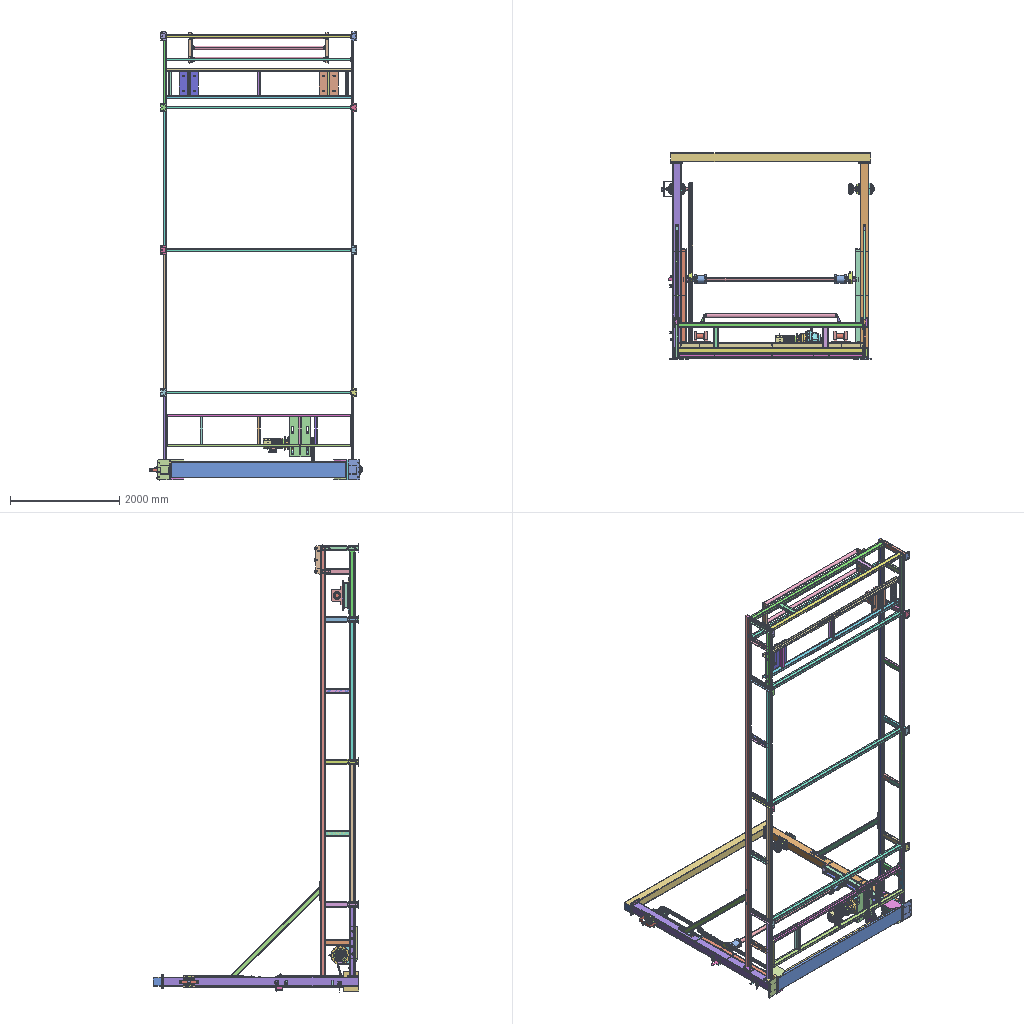Assembly | SolidWorks | 59 different items | 393 placed | box 3905 x 3772 x 8208 mm
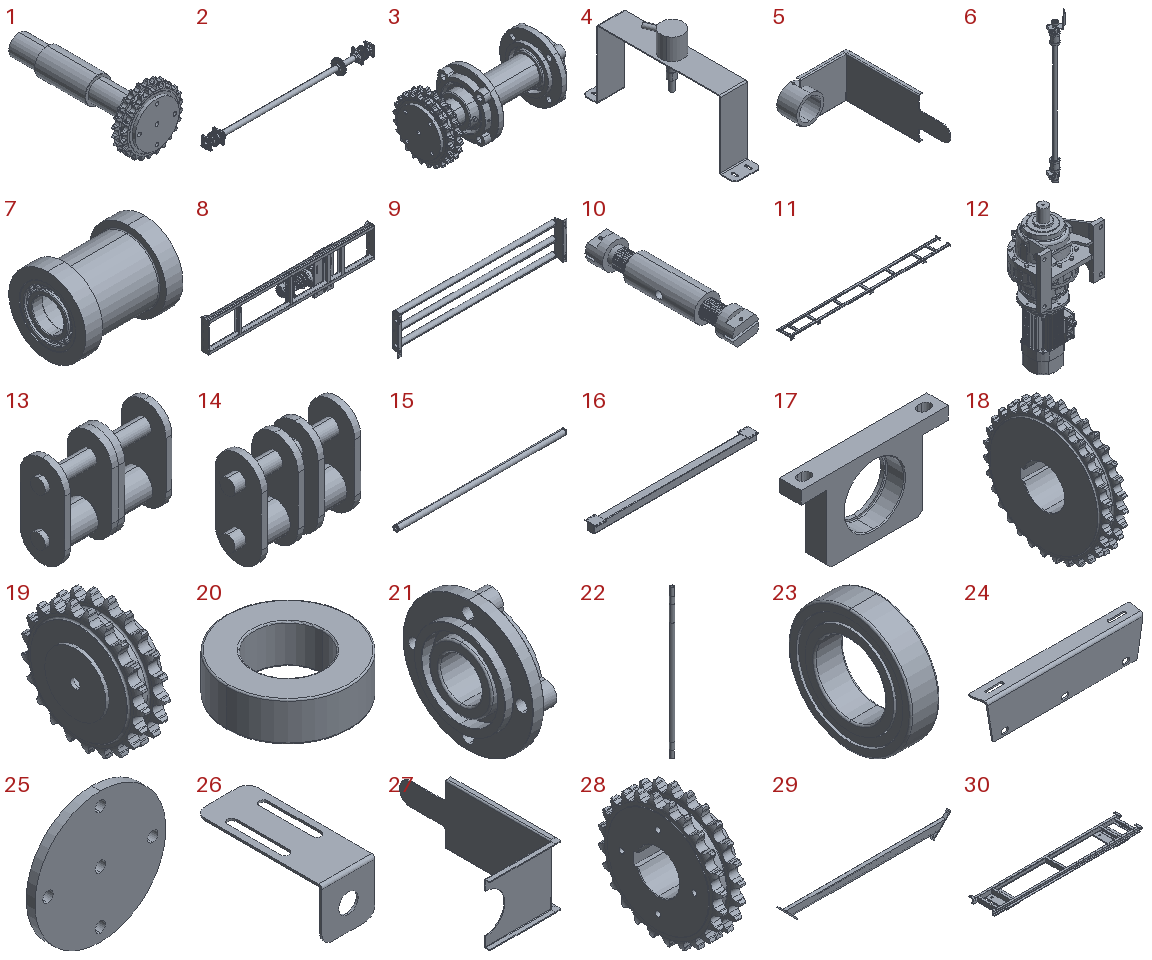Parts list (item | name | quantity | parent item | size | volume | features):
1 | (subassembly) | x2 | in 3 | 204.614 x 469.5 x 204.614 mm | 3507608 mm3 | -
2 | (subassembly) | x1 | - | 3215 x 262.517 x 262.783 mm | 19803434 mm3 | features ReferencePattern 3, MirrorCompFeat 1
3 | (subassembly) | x2 | - | 469.5 x 215 x 215 mm | 5837825 mm3 | -
4 | (subassembly) | x1 | - | 60 x 346 x 203 mm | 185638 mm3 | -
5 | (subassembly) | x1 | in 6 | 206.5 x 376.5 x 136 mm | 270788 mm3 | -
6 | (subassembly) | x1 | - | 288.692 x 309.852 x 3501 mm | 17816483 mm3 | features ReferencePattern 4, CompositeCurve 1, MirrorCompFeat 1
7 | (subassembly) | x2 | in 6 | 215 x 170 x 170 mm | 2119651 mm3 | features CompositeCurve 1
8 | (subassembly) | x1 | - | - | 58645223 mm3 | -
9 | (subassembly) | x1 | - | 2556 x 153 x 558.195 mm | 4678103 mm3 | features ReferencePattern 2, LocalLPattern 1
10 | (subassembly) | x1 | - | 75 x 420 x 75 mm | 1306901 mm3 | -
11 | - | x1 | - | 7924 x 758 x 126 mm | 27345410 mm3 | features MirrorStock 1
12 | - | x1 | in 8 | - | 37665619 mm3 | features BaseBody 24
13 | - | x148 | - | 62.7 x 24 x 49.4 mm | 23910 mm3 | features ICE 5, CombineBodies 2, Extrusion 1, MirrorSolid 1
14 | - | x148 | - | 62.7 x 24 x 49.4 mm | 23197 mm3 | features ICE 6, CombineBodies 1, Extrusion 1, MirrorSolid 1
15 | - | x3 | in 9 | 2449 x 76 x 76 mm | 1229105 mm3 | features Chamfer 4, ICE 3, Revolution 3, 3DProfileFeature 1, HoleWzd 1, MirrorPattern 1
16 | - | x1 | - | 3659 x 260 x 174 mm | 12792331 mm3 | features EndCap 2, HoleWzd 1, ICE 1, MirrorSolid 1, WeldMemberFeat 1, WeldmentFeature 1
17 | - | x4 | - | 344 x 50 x 190 mm | 1518259 mm3 | features ICE 3, Chamfer 2, Extrusion 1, Fillet 1
18 | - | x1 | in 2 | 70 x 262.456 x 262.787 mm | 2093366 mm3 | features Revolution 3, Chamfer 2, Cut 2, ICE 2, CirPattern 1, LPattern 1
19 | - | x1 | in 8 | 75 x 181.188 x 181.684 mm | 915452 mm3 | features ICE 11, Chamfer 4, Revolution 3, Cut 2, CirPattern 1, DelFace 1, LPattern 1
20 | - | x2 | in 6 | 125 x 125 x 39.7 mm | 333817 mm3 | features BaseBody 1
21 | - | x4 | in 3 | 75.4 x 215 x 215 mm | 1165108 mm3 | features Revolution 3, ICE 2, Fillet 1
22 | - | x1 | in 2 | 89 x 89 x 3215 mm | 11535395 mm3 | features ICE 9, MirrorPattern 2, Chamfer 1, Extrusion 1
23 | - | x4 | - | 33 x 140 x 140 mm | 264918 mm3 | features MBimport 1
24 | - | x2 | in 9 | 558.195 x 58.219 x 130 mm | 495394 mm3 | features ICE 2, LPattern 2, Fillet 1, FlatPattern 1, Gusset 1, SM3dBend 1, SMBaseFlange 1, SheetMetal 1
25 | - | x2 | in 1 | 150 x 10 x 150 mm | 171060 mm3 | features Extrusion 1, ICE 1
26 | - | x2 | - | 50 x 120 x 50 mm | 14154 mm3 | features ICE 2, Fillet 1, FlatPattern 1, SMBaseFlange 1, SheetMetal 1
27 | - | x1 | in 5 | 162 x 355 x 136 mm | 124416 mm3 | features ICE 3, EdgeFlange 2, Fillet 1, FlatPattern 1, SMBaseFlange 1, SheetMetal 1
28 | - | x4 | in 1, 2 | 70 x 204.614 x 204.614 mm | 1174386 mm3 | features Revolution 3, Chamfer 2, Cut 2, ICE 2, CirPattern 1, HoleWzd 1, LPattern 1
29 | - | x1 | - | 2475 x 48 x 257.387 mm | 3266090 mm3 | features ICE 2, MirrorSolid 1, WeldMemberFeat 1, WeldmentFeature 1
30 | - | x1 | - | 3487 x 660 x 134 mm | 19666004 mm3 | features ICE 2, LPattern 1, MirrorPattern 1, MoveCopyBody 1, WeldMemberFeat 1, WeldmentFeature 1
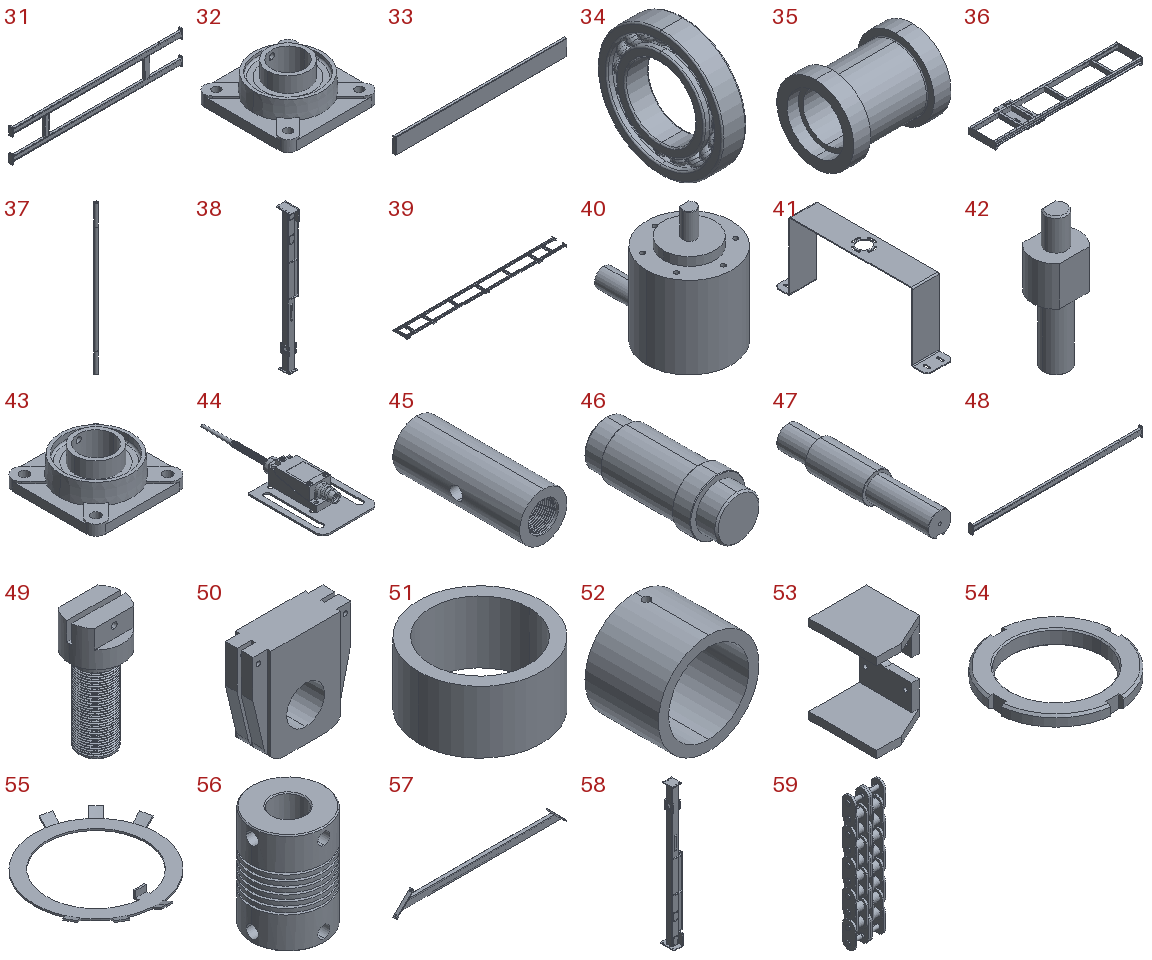31 | - | x1 | - | 3391 x 70 x 655 mm | 10020196 mm3 | features ICE 2, WeldMemberFeat 2, DelFace 1, MirrorSolid 1, MoveCopyBody 1, PLine 1, WeldCornerFeat 1, WeldmentFeature 1
32 | - | x2 | in 2 | 195 x 195 x 79.4 mm | 823685 mm3 | features Revolution 5, Boss 2, RevCut 2, CirPattern 1, Cut 1, Extrusion 1, RefAxis 1
33 | - | x1 | - | 3200 x 50 x 294 mm | 3763315 mm3 | features EdgeFlange 1, FlatPattern 1, SMBaseFlange 1, SheetMetal 1
34 | - | x4 | in 7 | 24 x 125 x 125 mm | 151869 mm3 | features Revolution 4, CirPattern 2, RefAxis 1, RevCut 1
35 | - | x2 | in 7 | 215 x 170 x 170 mm | 1815913 mm3 | features ICE 3, Cut 1, Extrusion 1, Fillet 1
36 | - | x1 | in 8 | 3390 x 776 x 160 mm | 20064178 mm3 | features ICE 7, MirrorSolid 2, Chamfer 1, MoveFace 1, WeldMemberFeat 1, WeldmentFeature 1
37 | - | x1 | in 6 | 76 x 76 x 3254 mm | 9186172 mm3 | features ICE 4, Chamfer 1, Extrusion 1, MirrorPattern 1
38 | - | x1 | - | 300 x 360 x 3598 mm | 23112152 mm3 | features ICE 40, MoveCopyBody 14, HoleWzd 8, MirrorSolid 7, MoveFace 7, LPattern 6, Gusset 4, CombineBodies 2, Fillet 2, Split 2, Cut 1, DelFace 1, WeldMemberFeat 1, WeldmentFeature 1
39 | - | x1 | - | 7924 x 758 x 126 mm | 27345410 mm3 | features ICE 7, WeldCornerFeat 4, WeldMemberFeat 2, LPattern 1, MoveCopyBody 1, WeldmentFeature 1
40 | - | x1 | in 4 | 50 x 75 x 68 mm | 100645 mm3 | features ICE 4, Chamfer 1, Extrusion 1
41 | - | x1 | in 4 | 60 x 346 x 155 mm | 74881 mm3 | features EdgeFlange 4, SMBaseFlange 2, Fillet 1, FlatPattern 1, ICE 1, MirrorPattern 1, SheetMetal 1
42 | - | x1 | in 4 | 18 x 14 x 52 mm | 5870 mm3 | features ICE 2, Chamfer 1, Extrusion 1
43 | - | x2 | in 2 | 213 x 213 x 84.3 mm | 1088893 mm3 | features Revolution 5, Boss 2, RevCut 2, CirPattern 1, Cut 1, Extrusion 1, RefAxis 1
44 | - | x2 | - | 75 x 198 x 27.9 mm | 57023 mm3 | features ICE 3, EdgeFlange 2, FlatPattern 2, SMBaseFlange 2, SheetMetal 2, BaseBody 1, Fillet 1
45 | - | x1 | in 10 | 75 x 200 x 75 mm | 538501 mm3 | features ICE 2, Extrusion 1, SweepThread 1
46 | - | x2 | - | 100 x 240 x 100 mm | 1475933 mm3 | features ICE 3, Chamfer 2, Extrusion 1
47 | - | x2 | in 1 | 89 x 459.5 x 89 mm | 2162162 mm3 | features ICE 3, HoleWzd 2, Chamfer 1, Extrusion 1, MoveFace 1
48 | - | x4 | - | 3391 x 70 x 180 mm | 4531337 mm3 | features ICE 2, MirrorSolid 1, PLine 1, WeldMemberFeat 1, WeldmentFeature 1
49 | - | x2 | in 10 | 75 x 75 x 170 mm | 384131 mm3 | features ICE 4, Chamfer 1, Extrusion 1, SweepThread 1
50 | - | x2 | in 6 | 180 x 65 x 180 mm | 1515776 mm3 | features ICE 4, Extrusion 1
51 | - | x2 | in 6 | 89 x 89 x 45 mm | 101788 mm3 | features Extrusion 1
52 | - | x2 | in 5, 6 | 89 x 65 x 89 mm | 146372 mm3 | features ICE 2, 3DProfileFeature 1, Extrusion 1, HoleWzd 1
53 | - | x2 | - | 236 x 277.5 x 360 mm | 5191315 mm3 | features Extrusion 1, ICE 1, MirrorSolid 1
54 | - | x2 | in 6 | 91.477 x 91.477 x 11 mm | 29647 mm3 | features Chamfer 3, CirPattern 1, Cut 1, Extrusion 1
55 | - | x2 | in 6 | 117.801 x 123.75 x 7 mm | 5903 mm3 | features Boss 1, Cut 1, Revolution 1
56 | - | x1 | in 4 | 18 x 18 x 25 mm | 4243 mm3 | features ICE 2, Chamfer 1, CirPattern 1, Extrusion 1, SweepCut 1
57 | - | x1 | - | 2475 x 48 x 257.387 mm | 3266090 mm3 | features MirrorStock 1
58 | - | x1 | - | 300 x 360 x 3598 mm | 23112152 mm3 | features MirrorStock 1
59 | - | x1 | - | 62.7 x 24 x 252.6 mm | 189611 mm3 | features ICE 7, Extrusion 1, Fillet 1, LPattern 1, MirrorPattern 1, MirrorSolid 1
Mates (type | each side: item.copy, entity, surface, feature):
In the top assembly
Coincident | 38.1 face plane Boss-Extrude21 | 39.1 face plane Boss-Extrude2
Concentric | 38.1 face cylinder Cut-Extrude4 | 47.1 face cylinder Boss-Extrude1
Coincident | 38.1 edge | 21.1 face plane Revolve1
Coincident | 38.1 face plane Boss-Extrude9 | 16.1 face plane Mirror1
Coincident | 17.1 face plane Boss-Extrude1 | 30.1 face plane Boss-Extrude3
Width | 17.1 face plane Boss-Extrude1 | 17.1 face plane Boss-Extrude1 | 30.1 face plane Boss-Extrude3 | 30.1 face plane Boss-Extrude3
Width | 53.1 face plane Boss-Extrude1 | 53.1 face plane Mirror2 | 38.1 face plane Boss-Extrude22 | 38.1 face plane Boss-Extrude22
Concentric | 46.1 face cylinder Cut-Extrude1 | 23.1 face cylinder Cylindrical Roller Bearing[NJ2216E].step<1>
Coincident | 46.1 face plane Cut-Extrude1 | 23.1 face plane Cylindrical Roller Bearing[NJ2216E].step<1>
Coincident | 46.1 face plane Cut-Extrude2 | 23.2 face plane Cylindrical Roller Bearing[NJ2216E].step<1>
Concentric | 46.1 face cylinder Cut-Extrude2 | 23.2 face cylinder Cylindrical Roller Bearing[NJ2216E].step<1>
Coincident | 17.1 face plane Cut-Extrude1 | 23.2 face plane Cylindrical Roller Bearing[NJ2216E].step<1>
Concentric | 23.1 face cylinder Cylindrical Roller Bearing[NJ2216E].step<1> | 17.2 face cylinder Cut-Extrude1
Coincident | 30.1 face plane Boss-Extrude3 | 17.2 face plane Boss-Extrude1
Concentric | 17.1 face cylinder Cut-Extrude1 | 23.2 face cylinder Cylindrical Roller Bearing[NJ2216E].step<1>
Coincident | 23.1 face plane Cylindrical Roller Bearing[NJ2216E].step<1> | 17.2 face plane Cut-Extrude1
Concentric | 38.1 face cylinder Cut-Extrude7 | 16.1 face cylinder Mirror1
Width | 59.1 face plane Mirror2 | 59.1 face plane LPattern2 | 50.1 face plane Cut-Extrude2 | 50.1 face plane Cut-Extrude2
Concentric | 50.1 face cylinder Cut-Extrude3 | 59.1 face cylinder Mirror2
Concentric | 59.1 face cylinder Mirror2 | 49.1 face cylinder Cut-Extrude3
Width | 49.1 face plane Cut-Extrude1 | 49.1 face plane Cut-Extrude1 | 59.1 face plane Mirror2 | 59.1 face plane Boss-Extrude2
Coincident | 38.1 face plane Boss-Extrude22 | 53.1 face plane Boss-Extrude1
Width | 38.1 face plane Boss-Extrude13 | 38.1 face plane Mirror5 | 20.1 face cylinder 3214A-2RSTN-HRB
Width | 33.1 face plane Edge-Flange1 | 33.1 face plane Edge-Flange1 | 53.2 face plane Mirror2 | 53.2 face plane Boss-Extrude1
Coincident | 58.1 face plane Column Symmetric End AA_Mirror | 33.1 face plane Base-Flange1
Coincident | 38.1 face plane Boss-Extrude24 | 29.1 face plane Mirror1
Coincident | 30.1 face plane LPattern1 | 39.1 face plane Gb/t707-1988 Hot-Rolled Channel 10(1)
Width | 39.1 face plane Boss-Extrude6 | 39.1 face plane Boss-Extrude6 | 38.1 face plane Gb/6728-1986 Square Hollow Section 160 X 160 X 5(1) | 38.1 face plane Gb/6728-1986 Square Hollow Section 160 X 160 X 5(1)
Coincident | 38.1 face plane Boss-Extrude26 | 39.1 face plane Boss-Extrude6
DistanceDim | 48.1 face plane Mirror3 | 39.1 face plane Gb/t707-1988 Hot-Rolled Channel 10(1)
Slot | 39.1 face cylinder Cut-Extrude1 | 30.1 face cylinder LPattern1
Coincident | 39.1 face plane Gb/t707-1988 Hot-Rolled Channel 10(6) | 48.2 face plane Mirror3
Width | 48.2 face plane Mirror3 | 48.2 face plane Mirror3 | 39.1 face plane Gb/t707-1988 Hot-Rolled Channel 10(6) | 39.1 face plane Gb/t707-1988 Hot-Rolled Channel 10(6)
Coincident | 39.1 face plane Gb/t707-1988 Hot-Rolled Channel 10(1) | 48.2 face plane Gb/t707-1988 Hot-Rolled Channel 10(1)
Coincident | 39.1 face plane Gb/t707-1988 Hot-Rolled Channel 10(6) | 48.3 face plane Mirror3
Coincident | 39.1 face plane Gb/t707-1988 Hot-Rolled Channel 10(6) | 48.4 face plane Mirror3
Coincident | 39.1 face plane Gb/t707-1988 Hot-Rolled Channel 10(1) | 48.4 face plane Gb/t707-1988 Hot-Rolled Channel 10(1)
Width | 48.4 face plane Mirror3 | 48.4 face plane Mirror3 | 39.1 face plane Gb/t707-1988 Hot-Rolled Channel 10(6) | 39.1 face plane Gb/t707-1988 Hot-Rolled Channel 10(6)
Coincident | 39.1 face plane Gb/t707-1988 Hot-Rolled Channel 10(1) | 48.3 face plane Gb/t707-1988 Hot-Rolled Channel 10(1)
Width | 48.3 face plane Mirror3 | 48.3 face plane Mirror3 | 39.1 face plane Gb/t707-1988 Hot-Rolled Channel 10(6) | 39.1 face plane Gb/t707-1988 Hot-Rolled Channel 10(6)
Coincident | 39.1 face plane Gb/t707-1988 Hot-Rolled Channel 10(1) | 31.1 face plane Mirror3
Width | 31.1 face plane Mirror3 | 31.1 face plane Mirror3 | 39.1 face plane Gb/t707-1988 Hot-Rolled Channel 10(1) | 39.1 face plane Gb/t707-1988 Hot-Rolled Channel 10(1)
DistanceDim | 31.1 face plane Gb/t707-1988 Hot-Rolled Channel 10(1) | 39.1 face plane Gb/t707-1988 Hot-Rolled Channel 10(1)
Coincident | 48.1 face plane Gb/t707-1988 Hot-Rolled Channel 10(1) | 31.1 face plane Gb/t707-1988 Hot-Rolled Channel 10(1)
Slot | 29.1 face plane Mirror1 | 38.1 face cylinder Boss-Extrude24
Coincident | 30.1 face plane Boss-Extrude2 | 39.1 face plane Gb/t707-1988 Hot-Rolled Channel 10(1)
DistanceDim | 17.1 face plane Boss-Extrude1 | 30.1 face plane Boss-Extrude3
Concentric | 32.1 face cylinder Base-Extrude | 58.1 face cylinder Column Symmetric End AA_Mirror | 2 times
Width | 22.1 face plane Boss-Extrude1 | 22.1 face plane Boss-Extrude1 | 38.1 face plane Gb/6728-1986 Square Hollow Section 160 X 160 X 5(1) | 58.1 face plane Column Symmetric End AA_Mirror
Width | 36.1 face plane Boss-Extrude2 | 36.1 face plane Mirror1 | 11.1 face plane End Face Side Brace_Mirror | 39.1 face plane Gb/t707-1988 Hot-Rolled Channel 10(1)
Slot | 36.1 face plane Cut-Extrude1 | 39.1 face cylinder Cut-Extrude4
Parallel | 36.1 face plane Boss-Extrude2 | 39.1 face plane Gb/t707-1988 Hot-Rolled Channel 10(1)
Width | 33.1 face plane Edge-Flange1 | 33.1 face plane Edge-Flange1 | 38.1 face plane Boss-Extrude22 | 58.1 face plane Column Symmetric End AA_Mirror
Concentric | 47.2 face cylinder Tap Drill for M10 Tap1 | 42.1 face cylinder Boss-Extrude3
Parallel | 58.1 face plane Column Symmetric End AA_Mirror | 41.1 face plane Base-Flange1
Coincident | 58.1 face plane Column Symmetric End AA_Mirror | 41.1 face plane Edge-Flange2
Coincident | 58.1 face plane Column Symmetric End AA_Mirror | 44.1 face plane Base-Flange1
Coincident | 58.1 face plane Column Symmetric End AA_Mirror | 26.1 face plane Base-Flange1
Parallel | 26.1 face plane Base-Flange1 | 44.1 face plane Base-Flange1
Parallel | 58.1 face plane Column Symmetric End AA_Mirror | 44.1 face plane Base-Flange1
Parallel | 26.2 face plane Base-Flange1 | 44.2 face plane Base-Flange1
Coincident | 26.2 face plane Base-Flange1 | 44.2 face plane Base-Flange1
Coincident | 58.1 face plane Column Symmetric End AA_Mirror | 26.2 face plane Base-Flange1
In subassembly 3
Concentric | 47.3 face cylinder Cut-Extrude2 | 21.2 face cylinder Revolve1
Concentric | 47.3 face cylinder Cut-Extrude1 | 21.3 face cylinder Revolve1
Coincident | 47.3 face plane Cut-Extrude1 | 21.3 face plane Revolve1
Concentric | 47.3 face cylinder Cut-Extrude1 | 3.1 face
Concentric | 21.2 face cylinder Boss-Extrude1 | 21.3 face cylinder Boss-Extrude1
Coincident | 47.3 face plane Cut-Extrude2 | 21.2 face plane Revolve1
In subassembly 1
Concentric | 47.4 face cylinder Cut-Extrude2 | 1.1 face
Coincident | 47.4 face plane Boss-Extrude1 | 1.1 face
Coincident | 47.4 face plane Cut-Extrude3 | 1.1 face
Concentric | 47.4 face cylinder Cut-Extrude2 | 25.1 face cylinder Boss-Extrude1
Concentric | 1.1 face | 25.1 face cylinder Cut-Extrude1
Coincident | 1.1 face | 25.1 face plane Boss-Extrude1
Concentric | 47.4 face cylinder Cut-Extrude2 | 28.1 face cylinder Revolve1
Coincident | 25.1 face plane Boss-Extrude1 | 28.1 face plane Revolve1
Coincident | 47.4 face plane Boss-Extrude1 | 28.1 face plane Revolve1
In subassembly 6
Concentric | 37.1 face cylinder Cut-Extrude2 | 35.1 face cylinder Cut-Extrude1
Concentric | 37.1 face cylinder Cut-Extrude2 | 51.1 face cylinder Boss-Extrude1
Concentric | 37.1 face cylinder Cut-Extrude2 | 50.2 face cylinder Cut-Extrude1
Coincident | 51.1 face plane Boss-Extrude1 | 50.2 face plane Boss-Extrude1
Concentric | 37.1 face cylinder Cut-Extrude2 | 52.1 face cylinder Boss-Extrude1
Concentric | 37.1 face cylinder Cut-Extrude1 | 55.1 face cylinder Cut-Extrude2
Concentric | 37.1 face cylinder Cut-Extrude1 | 54.1 face cylinder Base-Extrude
Coincident | 55.1 face plane Base-Revolve | 54.1 face plane Base-Extrude
Concentric | 37.1 face cylinder Cut-Extrude2 | 55.2 face cylinder Cut-Extrude2
Concentric | 37.1 face cylinder Cut-Extrude2 | 54.2 face cylinder Base-Extrude
Coincident | 55.2 face plane Base-Revolve | 54.2 face plane Base-Extrude
Concentric | 37.1 face cylinder Cut-Extrude2 | 52.2 face cylinder Boss-Extrude1
Coincident | 50.2 face plane Boss-Extrude1 | 52.2 face plane Boss-Extrude1
Coincident | 52.1 face plane Boss-Extrude1 | 50.3 face plane Boss-Extrude1
Coincident | 35.1 face plane Boss-Extrude1 | 51.1 face plane Boss-Extrude1
Concentric | 37.1 face cylinder Cut-Extrude2 | 20.2 face cylinder 3214A-2RSTN-HRB
Coincident | 37.1 face plane Cut-Extrude2 | 34.1 face plane Revolve1
Coincident | 52.1 face plane Boss-Extrude1 | 20.3 face plane 3214A-2RSTN-HRB
Coincident | 55.2 face plane Base-Revolve | 20.2 face plane 3214A-2RSTN-HRB
Coincident | 52.2 face plane Boss-Extrude1 | 20.2 face plane 3214A-2RSTN-HRB
Coincident | 55.1 face plane Base-Revolve | 20.3 face plane 3214A-2RSTN-HRB
In subassembly 7
Concentric | 35.2 face cylinder Cut-Extrude2 | 34.2 face cylinder Revolve1
Coincident | 35.2 face plane Cut-Extrude2 | 34.2 face plane Revolve1
Concentric | 35.2 face cylinder Cut-Extrude3 | 34.3 face cylinder Revolve1
Coincident | 35.2 face plane Cut-Extrude3 | 34.3 face plane Revolve1
In subassembly 5
Width | 27.1 face plane Base-Flange1 | 27.1 face plane Base-Flange1 | 52.1 face plane Boss-Extrude1 | 52.1 face plane Boss-Extrude1
Concentric | 52.1 face cylinder Boss-Extrude1 | 27.1 face cylinder Base-Flange1
In subassembly 2
Coincident | 22.2 face plane Mirror1 | 28.1 face plane Revolve1
Concentric | 22.2 face cylinder Cut-Extrude3 | 18.1 face cylinder Revolve2
Coincident | 22.2 face plane Cut-Extrude3 | 18.1 face plane Revolve2
Concentric | 22.2 face cylinder Mirror1 | 32.2 face cylinder Boss-Revolve4
Concentric | 22.2 face cylinder Mirror1 | 43.1 face cylinder Boss-Revolve4
Parallel | 32.2 face plane Base-Extrude | 43.1 face plane Base-Extrude
Coincident | 22.2 face plane Mirror1 | 43.1 face plane Boss-Revolve4
Concentric | 22.2 face cylinder Mirror1 | 28.1 face cylinder Revolve1
Coincident | 22.2 face plane Boss-Extrude1 | 32.3 face plane Base-Extrude
In subassembly 8
Concentric | 12.1 face cylinder Open CASCADE STEP translator 7.6 69.1-1/Open CASCADE STEP translator 7.6 69.1.1-1/Open CASCADE STEP translator 7.6 69.1.1.1-1-solid1 | 19.1 face cylinder Cut-Extrude7
Coincident | 12.1 face plane Open CASCADE STEP translator 7.6 69.1-1/Open CASCADE STEP translator 7.6 69.1.1-1/Open CASCADE STEP translator 7.6 69.1.1.1-1-solid1 | 19.1 face plane Revolve1
Coincident | 36.2 face plane Boss-Extrude1 | 12.1 face plane Open CASCADE STEP translator 7.6 69.1-1/Open CASCADE STEP translator 7.6 69.1.1-1/Open CASCADE STEP translator 7.6 69.1.1.1-1-solid1
Slot | 12.1 face cylinder Open CASCADE STEP translator 7.6 69.1-1/Open CASCADE STEP translator 7.6 69.1.1-1/Open CASCADE STEP translator 7.6 69.1.1.1-1-solid1 | 36.2 face plane Boss-Extrude1 | 2 times
In subassembly 9
Coincident | 15.1 face plane Revolve3 | 24.1 face plane Base-Flange1
Concentric | 24.1 face cylinder LPattern5 | 15.1 face cylinder Revolve3
Parallel | 24.1 face plane LPattern5 | 15.1 face plane Cut-Extrude3
Concentric | 15.1 face cylinder Revolve3 | 24.2 face cylinder LPattern5
Coincident | 15.1 face plane Revolve3 | 24.2 face plane Base-Flange1
Parallel | 15.1 face plane Cut-Extrude3 | 24.2 face plane LPattern5
In subassembly 10
Concentric | 45.1 face cylinder Boss-Extrude1 | 49.2 face cylinder Boss-Extrude1
DistanceDim | 49.2 face plane Boss-Extrude1 | 45.1 face plane Boss-Extrude1
Concentric | 45.1 face cylinder Boss-Extrude1 | 49.3 face cylinder Boss-Extrude1
Coincident | 49.2 face plane Cut-Extrude1 | 49.3 face plane Cut-Extrude1
DistanceDim | 49.3 face plane Boss-Extrude1 | 45.1 face plane Boss-Extrude1
In subassembly 4
Concentric | 41.2 face cylinder Base-Flange1 | 40.1 face cylinder Boss-Extrude2
Coincident | 41.2 face plane Base-Flange1 | 40.1 face plane Boss-Extrude1
Concentric | 40.1 face cylinder Boss-Extrude3 | 56.1 face cylinder Cut-Extrude2
DistanceDim | 56.1 face plane Boss-Extrude1 | 40.1 face plane Boss-Extrude2
Concentric | 56.1 face cylinder Cut-Extrude2 | 42.2 face cylinder Boss-Extrude1
DistanceDim | 42.2 face plane Boss-Extrude2 | 56.1 face plane Boss-Extrude1